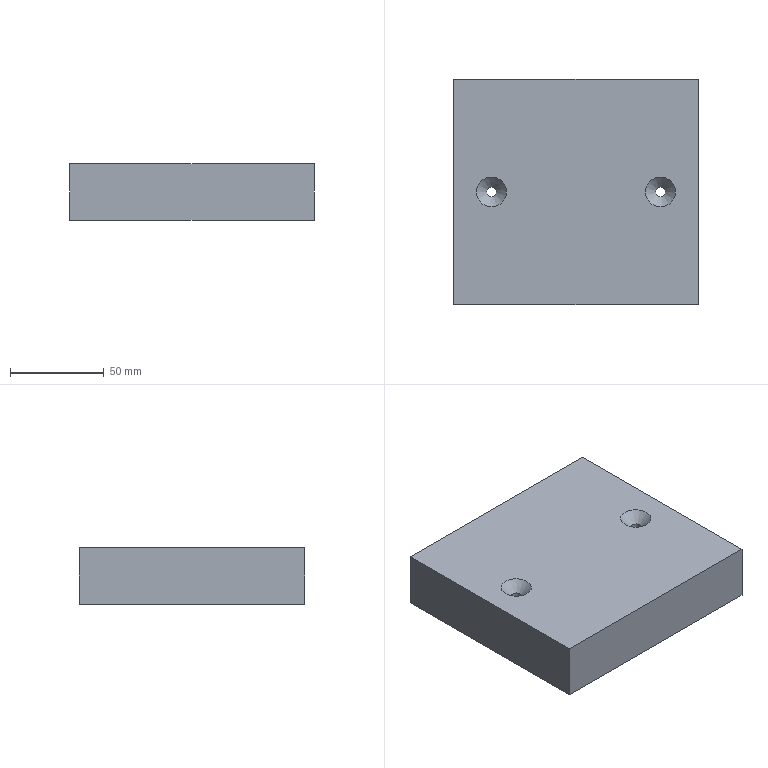Part | STEP file | YBQDJ-YY-5 | 1 solid | 10 faces | box 130 x 120 x 30 mm | volume 465920 mm3 | plane 6 | cylinder 2 | cone 2 | commonest cylinder face diameters 5.2 x2
STEP:
#1=CARTESIAN_POINT('',(0.,0.,0.));
#2=DIRECTION('',(0.,0.,1.));
#3=DIRECTION('',(1.,0.,0.));
#4=AXIS2_PLACEMENT_3D('',#1,#2,#3);
#5=CARTESIAN_POINT('',(168.9,305.,150.));
#6=VERTEX_POINT('',#5);
#7=CARTESIAN_POINT('',(171.5,305.,150.));
#8=DIRECTION('',(0.,0.,-1.));
#9=DIRECTION('',(-1.,0.,0.));
#10=AXIS2_PLACEMENT_3D('',#7,#8,#9);
#11=CIRCLE('',#10,2.6);
#12=CARTESIAN_POINT('',(171.5,305.,200.5));
#13=DIRECTION('',(0.,0.,-1.));
#14=DIRECTION('',(1.,0.,0.));
#15=AXIS2_PLACEMENT_3D('',#12,#13,#14);
#16=CYLINDRICAL_SURFACE('',#15,2.6);
#17=CARTESIAN_POINT('',(3.142,50.5));
#18=DIRECTION('',(1.,0.));
#19=VECTOR('',#18,1.);
#20=LINE('',#17,#19);
#21=(GEOMETRIC_REPRESENTATION_CONTEXT(2)PARAMETRIC_REPRESENTATION_CONTEXT()REPRESENTATION_CONTEXT('',''));
#22=DEFINITIONAL_REPRESENTATION('',(#20),#21);
#23=PCURVE('',#16,#22);
#24=CARTESIAN_POINT('',(251.5,412.,150.));
#25=DIRECTION('',(0.,0.,-1.));
#26=DIRECTION('',(-1.,0.,0.));
#27=AXIS2_PLACEMENT_3D('',#24,#25,#26);
#28=PLANE('',#27);
#29=CARTESIAN_POINT('',(80.,-107.));
#30=DIRECTION('',(1.,0.));
#31=AXIS2_PLACEMENT_2D('',#29,#30);
#32=CIRCLE('',#31,2.6);
#33=(GEOMETRIC_REPRESENTATION_CONTEXT(2)PARAMETRIC_REPRESENTATION_CONTEXT()REPRESENTATION_CONTEXT('',''));
#34=DEFINITIONAL_REPRESENTATION('',(#32),#33);
#35=PCURVE('',#28,#34);
#36=SURFACE_CURVE('',#11,(#23,#35),.PCURVE_S1.);
#37=EDGE_CURVE('',#6,#6,#36,.T.);
#38=ORIENTED_EDGE('',*,*,#37,.F.);
#39=CARTESIAN_POINT('',(168.9,305.,174.6));
#40=VERTEX_POINT('',#39);
#41=CARTESIAN_POINT('',(168.9,305.,174.6));
#42=CARTESIAN_POINT('',(168.9,305.,150.));
#43=B_SPLINE_CURVE_WITH_KNOTS('',1,(#41,#42),.UNSPECIFIED.,.F.,.F.,(2,2),(25.9,50.5),.PIECEWISE_BEZIER_KNOTS.);
#44=CARTESIAN_POINT('',(3.142,0.));
#45=DIRECTION('',(0.,1.));
#46=VECTOR('',#45,1.);
#47=LINE('',#44,#46);
#48=(GEOMETRIC_REPRESENTATION_CONTEXT(2)PARAMETRIC_REPRESENTATION_CONTEXT()REPRESENTATION_CONTEXT('',''));
#49=DEFINITIONAL_REPRESENTATION('',(#47),#48);
#50=PCURVE('',#16,#49);
#51=CARTESIAN_POINT('',(9.425,0.));
#52=DIRECTION('',(0.,1.));
#53=VECTOR('',#52,1.);
#54=LINE('',#51,#53);
#55=(GEOMETRIC_REPRESENTATION_CONTEXT(2)PARAMETRIC_REPRESENTATION_CONTEXT()REPRESENTATION_CONTEXT('',''));
#56=DEFINITIONAL_REPRESENTATION('',(#54),#55);
#57=PCURVE('',#16,#56);
#58=SEAM_CURVE('',#43,(#50,#57),.PCURVE_S1.);
#59=EDGE_CURVE('',#40,#6,#58,.T.);
#60=ORIENTED_EDGE('',*,*,#59,.F.);
#61=CARTESIAN_POINT('',(171.5,305.,174.6));
#62=DIRECTION('',(0.,0.,1.));
#63=DIRECTION('',(-1.,0.,0.));
#64=AXIS2_PLACEMENT_3D('',#61,#62,#63);
#65=CIRCLE('',#64,2.6);
#66=CARTESIAN_POINT('',(9.425,25.9));
#67=DIRECTION('',(-1.,0.));
#68=VECTOR('',#67,1.);
#69=LINE('',#66,#68);
#70=(GEOMETRIC_REPRESENTATION_CONTEXT(2)PARAMETRIC_REPRESENTATION_CONTEXT()REPRESENTATION_CONTEXT('',''));
#71=DEFINITIONAL_REPRESENTATION('',(#69),#70);
#72=PCURVE('',#16,#71);
#73=CARTESIAN_POINT('',(171.5,305.,175.));
#74=DIRECTION('',(0.,0.,1.));
#75=DIRECTION('',(-1.,0.,0.));
#76=AXIS2_PLACEMENT_3D('',#73,#74,#75);
#77=CONICAL_SURFACE('',#76,3.,0.7854);
#78=CARTESIAN_POINT('',(0.,-0.4));
#79=DIRECTION('',(1.,0.));
#80=VECTOR('',#79,1.);
#81=LINE('',#78,#80);
#82=(GEOMETRIC_REPRESENTATION_CONTEXT(2)PARAMETRIC_REPRESENTATION_CONTEXT()REPRESENTATION_CONTEXT('',''));
#83=DEFINITIONAL_REPRESENTATION('',(#81),#82);
#84=PCURVE('',#77,#83);
#85=SURFACE_CURVE('',#65,(#72,#84),.PCURVE_S1.);
#86=EDGE_CURVE('',#40,#40,#85,.T.);
#87=ORIENTED_EDGE('',*,*,#86,.F.);
#88=ORIENTED_EDGE('',*,*,#59,.T.);
#89=EDGE_LOOP('',(#38,#60,#87,#88));
#90=FACE_BOUND('',#89,.F.);
#91=ADVANCED_FACE('',(#90),#16,.F.);
#92=ORIENTED_EDGE('',*,*,#86,.T.);
#93=CARTESIAN_POINT('',(163.5,305.,180.));
#94=VERTEX_POINT('',#93);
#95=CARTESIAN_POINT('',(168.9,305.,174.6));
#96=CARTESIAN_POINT('',(163.5,305.,180.));
#97=B_SPLINE_CURVE_WITH_KNOTS('',1,(#95,#96),.UNSPECIFIED.,.F.,.F.,(2,2),(-0.5657,7.071),.PIECEWISE_BEZIER_KNOTS.);
#98=CARTESIAN_POINT('',(6.283,0.));
#99=DIRECTION('',(0.,1.));
#100=VECTOR('',#99,1.);
#101=LINE('',#98,#100);
#102=(GEOMETRIC_REPRESENTATION_CONTEXT(2)PARAMETRIC_REPRESENTATION_CONTEXT()REPRESENTATION_CONTEXT('',''));
#103=DEFINITIONAL_REPRESENTATION('',(#101),#102);
#104=PCURVE('',#77,#103);
#105=CARTESIAN_POINT('',(0.,0.));
#106=DIRECTION('',(0.,1.));
#107=VECTOR('',#106,1.);
#108=LINE('',#105,#107);
#109=(GEOMETRIC_REPRESENTATION_CONTEXT(2)PARAMETRIC_REPRESENTATION_CONTEXT()REPRESENTATION_CONTEXT('',''));
#110=DEFINITIONAL_REPRESENTATION('',(#108),#109);
#111=PCURVE('',#77,#110);
#112=SEAM_CURVE('',#97,(#104,#111),.PCURVE_S1.);
#113=EDGE_CURVE('',#40,#94,#112,.T.);
#114=ORIENTED_EDGE('',*,*,#113,.T.);
#115=CARTESIAN_POINT('',(179.5,305.,180.));
#116=VERTEX_POINT('',#115);
#117=CARTESIAN_POINT('',(171.5,305.,180.));
#118=DIRECTION('',(0.,0.,-1.));
#119=DIRECTION('',(1.,0.,0.));
#120=AXIS2_PLACEMENT_3D('',#117,#118,#119);
#121=CIRCLE('',#120,8.);
#122=CARTESIAN_POINT('',(9.425,5.));
#123=DIRECTION('',(-1.,0.));
#124=VECTOR('',#123,1.);
#125=LINE('',#122,#124);
#126=(GEOMETRIC_REPRESENTATION_CONTEXT(2)PARAMETRIC_REPRESENTATION_CONTEXT()REPRESENTATION_CONTEXT('',''));
#127=DEFINITIONAL_REPRESENTATION('',(#125),#126);
#128=PCURVE('',#77,#127);
#129=CARTESIAN_POINT('',(-49.497,0.,180.));
#130=DIRECTION('',(0.,0.,1.));
#131=DIRECTION('',(1.,0.,0.));
#132=AXIS2_PLACEMENT_3D('',#129,#130,#131);
#133=PLANE('',#132);
#134=CARTESIAN_POINT('',(228.997,305.));
#135=CARTESIAN_POINT('',(228.997,291.144));
#136=CARTESIAN_POINT('',(216.997,298.072));
#137=CARTESIAN_POINT('',(204.997,305.));
#138=CARTESIAN_POINT('',(216.997,311.928));
#139=CARTESIAN_POINT('',(228.997,318.856));
#140=CARTESIAN_POINT('',(228.997,305.));
#141=(BOUNDED_CURVE()B_SPLINE_CURVE(2,(#134,#135,#136,#137,#138,#139,#140),.UNSPECIFIED.,.T.,.F.)B_SPLINE_CURVE_WITH_KNOTS((1,2,2,2,2,1),(-2.094,0.,2.094,4.189,6.283,8.378),.UNSPECIFIED.)CURVE()GEOMETRIC_REPRESENTATION_ITEM()RATIONAL_B_SPLINE_CURVE((1.,0.5,1.,0.5,1.,0.5,1.))REPRESENTATION_ITEM(''));
#142=(GEOMETRIC_REPRESENTATION_CONTEXT(2)PARAMETRIC_REPRESENTATION_CONTEXT()REPRESENTATION_CONTEXT('',''));
#143=DEFINITIONAL_REPRESENTATION('',(#141),#142);
#144=PCURVE('',#133,#143);
#145=SURFACE_CURVE('',#121,(#128,#144),.PCURVE_S1.);
#146=EDGE_CURVE('',#94,#116,#145,.T.);
#147=ORIENTED_EDGE('',*,*,#146,.T.);
#148=CARTESIAN_POINT('',(171.5,305.,180.));
#149=DIRECTION('',(0.,0.,-1.));
#150=DIRECTION('',(1.,0.,0.));
#151=AXIS2_PLACEMENT_3D('',#148,#149,#150);
#152=CIRCLE('',#151,8.);
#153=CARTESIAN_POINT('',(3.142,5.));
#154=DIRECTION('',(-1.,0.));
#155=VECTOR('',#154,1.);
#156=LINE('',#153,#155);
#157=(GEOMETRIC_REPRESENTATION_CONTEXT(2)PARAMETRIC_REPRESENTATION_CONTEXT()REPRESENTATION_CONTEXT('',''));
#158=DEFINITIONAL_REPRESENTATION('',(#156),#157);
#159=PCURVE('',#77,#158);
#160=CARTESIAN_POINT('',(228.997,305.));
#161=CARTESIAN_POINT('',(228.997,291.144));
#162=CARTESIAN_POINT('',(216.997,298.072));
#163=CARTESIAN_POINT('',(204.997,305.));
#164=CARTESIAN_POINT('',(216.997,311.928));
#165=CARTESIAN_POINT('',(228.997,318.856));
#166=CARTESIAN_POINT('',(228.997,305.));
#167=(BOUNDED_CURVE()B_SPLINE_CURVE(2,(#160,#161,#162,#163,#164,#165,#166),.UNSPECIFIED.,.T.,.F.)B_SPLINE_CURVE_WITH_KNOTS((1,2,2,2,2,1),(-2.094,0.,2.094,4.189,6.283,8.378),.UNSPECIFIED.)CURVE()GEOMETRIC_REPRESENTATION_ITEM()RATIONAL_B_SPLINE_CURVE((1.,0.5,1.,0.5,1.,0.5,1.))REPRESENTATION_ITEM(''));
#168=(GEOMETRIC_REPRESENTATION_CONTEXT(2)PARAMETRIC_REPRESENTATION_CONTEXT()REPRESENTATION_CONTEXT('',''));
#169=DEFINITIONAL_REPRESENTATION('',(#167),#168);
#170=PCURVE('',#133,#169);
#171=SURFACE_CURVE('',#152,(#159,#170),.PCURVE_S1.);
#172=EDGE_CURVE('',#116,#94,#171,.T.);
#173=ORIENTED_EDGE('',*,*,#172,.T.);
#174=ORIENTED_EDGE('',*,*,#113,.F.);
#175=EDGE_LOOP('',(#92,#114,#147,#173,#174));
#176=FACE_BOUND('',#175,.F.);
#177=ADVANCED_FACE('',(#176),#77,.F.);
#178=CARTESIAN_POINT('',(258.9,305.,150.));
#179=VERTEX_POINT('',#178);
#180=CARTESIAN_POINT('',(261.5,305.,150.));
#181=DIRECTION('',(0.,0.,-1.));
#182=DIRECTION('',(-1.,0.,0.));
#183=AXIS2_PLACEMENT_3D('',#180,#181,#182);
#184=CIRCLE('',#183,2.6);
#185=CARTESIAN_POINT('',(261.5,305.,200.5));
#186=DIRECTION('',(0.,0.,-1.));
#187=DIRECTION('',(-1.,0.,0.));
#188=AXIS2_PLACEMENT_3D('',#185,#186,#187);
#189=CYLINDRICAL_SURFACE('',#188,2.6);
#190=CARTESIAN_POINT('',(0.,50.5));
#191=DIRECTION('',(1.,0.));
#192=VECTOR('',#191,1.);
#193=LINE('',#190,#192);
#194=(GEOMETRIC_REPRESENTATION_CONTEXT(2)PARAMETRIC_REPRESENTATION_CONTEXT()REPRESENTATION_CONTEXT('',''));
#195=DEFINITIONAL_REPRESENTATION('',(#193),#194);
#196=PCURVE('',#189,#195);
#197=CARTESIAN_POINT('',(-10.,-107.));
#198=DIRECTION('',(1.,0.));
#199=AXIS2_PLACEMENT_2D('',#197,#198);
#200=CIRCLE('',#199,2.6);
#201=(GEOMETRIC_REPRESENTATION_CONTEXT(2)PARAMETRIC_REPRESENTATION_CONTEXT()REPRESENTATION_CONTEXT('',''));
#202=DEFINITIONAL_REPRESENTATION('',(#200),#201);
#203=PCURVE('',#28,#202);
#204=SURFACE_CURVE('',#184,(#196,#203),.PCURVE_S1.);
#205=EDGE_CURVE('',#179,#179,#204,.T.);
#206=ORIENTED_EDGE('',*,*,#205,.F.);
#207=CARTESIAN_POINT('',(258.9,305.,174.6));
#208=VERTEX_POINT('',#207);
#209=CARTESIAN_POINT('',(258.9,305.,174.6));
#210=CARTESIAN_POINT('',(258.9,305.,150.));
#211=B_SPLINE_CURVE_WITH_KNOTS('',1,(#209,#210),.UNSPECIFIED.,.F.,.F.,(2,2),(25.9,50.5),.PIECEWISE_BEZIER_KNOTS.);
#212=CARTESIAN_POINT('',(0.,0.));
#213=DIRECTION('',(0.,1.));
#214=VECTOR('',#213,1.);
#215=LINE('',#212,#214);
#216=(GEOMETRIC_REPRESENTATION_CONTEXT(2)PARAMETRIC_REPRESENTATION_CONTEXT()REPRESENTATION_CONTEXT('',''));
#217=DEFINITIONAL_REPRESENTATION('',(#215),#216);
#218=PCURVE('',#189,#217);
#219=CARTESIAN_POINT('',(6.283,0.));
#220=DIRECTION('',(0.,1.));
#221=VECTOR('',#220,1.);
#222=LINE('',#219,#221);
#223=(GEOMETRIC_REPRESENTATION_CONTEXT(2)PARAMETRIC_REPRESENTATION_CONTEXT()REPRESENTATION_CONTEXT('',''));
#224=DEFINITIONAL_REPRESENTATION('',(#222),#223);
#225=PCURVE('',#189,#224);
#226=SEAM_CURVE('',#211,(#218,#225),.PCURVE_S1.);
#227=EDGE_CURVE('',#208,#179,#226,.T.);
#228=ORIENTED_EDGE('',*,*,#227,.F.);
#229=CARTESIAN_POINT('',(264.1,305.,174.6));
#230=VERTEX_POINT('',#229);
#231=CARTESIAN_POINT('',(261.5,305.,174.6));
#232=DIRECTION('',(0.,0.,1.));
#233=DIRECTION('',(1.,0.,0.));
#234=AXIS2_PLACEMENT_3D('',#231,#232,#233);
#235=CIRCLE('',#234,2.6);
#236=CARTESIAN_POINT('',(3.142,25.9));
#237=DIRECTION('',(-1.,0.));
#238=VECTOR('',#237,1.);
#239=LINE('',#236,#238);
#240=(GEOMETRIC_REPRESENTATION_CONTEXT(2)PARAMETRIC_REPRESENTATION_CONTEXT()REPRESENTATION_CONTEXT('',''));
#241=DEFINITIONAL_REPRESENTATION('',(#239),#240);
#242=PCURVE('',#189,#241);
#243=CARTESIAN_POINT('',(261.5,305.,175.));
#244=DIRECTION('',(0.,0.,1.));
#245=DIRECTION('',(1.,0.,0.));
#246=AXIS2_PLACEMENT_3D('',#243,#244,#245);
#247=CONICAL_SURFACE('',#246,3.,0.7854);
#248=CARTESIAN_POINT('',(0.,-0.4));
#249=DIRECTION('',(1.,0.));
#250=VECTOR('',#249,1.);
#251=LINE('',#248,#250);
#252=(GEOMETRIC_REPRESENTATION_CONTEXT(2)PARAMETRIC_REPRESENTATION_CONTEXT()REPRESENTATION_CONTEXT('',''));
#253=DEFINITIONAL_REPRESENTATION('',(#251),#252);
#254=PCURVE('',#247,#253);
#255=SURFACE_CURVE('',#235,(#242,#254),.PCURVE_S1.);
#256=EDGE_CURVE('',#230,#208,#255,.T.);
#257=ORIENTED_EDGE('',*,*,#256,.F.);
#258=CARTESIAN_POINT('',(261.5,305.,174.6));
#259=DIRECTION('',(0.,0.,1.));
#260=DIRECTION('',(1.,0.,0.));
#261=AXIS2_PLACEMENT_3D('',#258,#259,#260);
#262=CIRCLE('',#261,2.6);
#263=CARTESIAN_POINT('',(9.425,25.9));
#264=DIRECTION('',(-1.,0.));
#265=VECTOR('',#264,1.);
#266=LINE('',#263,#265);
#267=(GEOMETRIC_REPRESENTATION_CONTEXT(2)PARAMETRIC_REPRESENTATION_CONTEXT()REPRESENTATION_CONTEXT('',''));
#268=DEFINITIONAL_REPRESENTATION('',(#266),#267);
#269=PCURVE('',#189,#268);
#270=CARTESIAN_POINT('',(0.,-0.4));
#271=DIRECTION('',(1.,0.));
#272=VECTOR('',#271,1.);
#273=LINE('',#270,#272);
#274=(GEOMETRIC_REPRESENTATION_CONTEXT(2)PARAMETRIC_REPRESENTATION_CONTEXT()REPRESENTATION_CONTEXT('',''));
#275=DEFINITIONAL_REPRESENTATION('',(#273),#274);
#276=PCURVE('',#247,#275);
#277=SURFACE_CURVE('',#262,(#269,#276),.PCURVE_S1.);
#278=EDGE_CURVE('',#208,#230,#277,.T.);
#279=ORIENTED_EDGE('',*,*,#278,.F.);
#280=ORIENTED_EDGE('',*,*,#227,.T.);
#281=EDGE_LOOP('',(#206,#228,#257,#279,#280));
#282=FACE_BOUND('',#281,.F.);
#283=ADVANCED_FACE('',(#282),#189,.F.);
#284=CARTESIAN_POINT('',(281.5,365.,180.));
#285=VERTEX_POINT('',#284);
#286=CARTESIAN_POINT('',(151.5,365.,180.));
#287=VERTEX_POINT('',#286);
#288=CARTESIAN_POINT('',(-49.497,365.,180.));
#289=DIRECTION('',(-1.,0.,0.));
#290=VECTOR('',#289,1.);
#291=LINE('',#288,#290);
#292=CARTESIAN_POINT('',(276.5,365.,157.5));
#293=DIRECTION('',(0.,1.,0.));
#294=DIRECTION('',(0.,0.,1.));
#295=AXIS2_PLACEMENT_3D('',#292,#293,#294);
#296=PLANE('',#295);
#297=CARTESIAN_POINT('',(22.5,-325.997));
#298=DIRECTION('',(0.,-1.));
#299=VECTOR('',#298,1.);
#300=LINE('',#297,#299);
#301=(GEOMETRIC_REPRESENTATION_CONTEXT(2)PARAMETRIC_REPRESENTATION_CONTEXT()REPRESENTATION_CONTEXT('',''));
#302=DEFINITIONAL_REPRESENTATION('',(#300),#301);
#303=PCURVE('',#296,#302);
#304=CARTESIAN_POINT('',(0.,365.));
#305=DIRECTION('',(-1.,0.));
#306=VECTOR('',#305,1.);
#307=LINE('',#304,#306);
#308=(GEOMETRIC_REPRESENTATION_CONTEXT(2)PARAMETRIC_REPRESENTATION_CONTEXT()REPRESENTATION_CONTEXT('',''));
#309=DEFINITIONAL_REPRESENTATION('',(#307),#308);
#310=PCURVE('',#133,#309);
#311=SURFACE_CURVE('',#291,(#303,#310),.PCURVE_S1.);
#312=EDGE_CURVE('',#285,#287,#311,.T.);
#313=ORIENTED_EDGE('',*,*,#312,.F.);
#314=CARTESIAN_POINT('',(281.5,365.,150.));
#315=VERTEX_POINT('',#314);
#316=CARTESIAN_POINT('',(281.5,365.,185.));
#317=DIRECTION('',(0.,0.,1.));
#318=VECTOR('',#317,1.);
#319=LINE('',#316,#318);
#320=CARTESIAN_POINT('',(27.5,5.));
#321=DIRECTION('',(1.,0.));
#322=VECTOR('',#321,1.);
#323=LINE('',#320,#322);
#324=(GEOMETRIC_REPRESENTATION_CONTEXT(2)PARAMETRIC_REPRESENTATION_CONTEXT()REPRESENTATION_CONTEXT('',''));
#325=DEFINITIONAL_REPRESENTATION('',(#323),#324);
#326=PCURVE('',#296,#325);
#327=CARTESIAN_POINT('',(281.5,210.,185.));
#328=DIRECTION('',(-1.,0.,0.));
#329=DIRECTION('',(0.,-1.,0.));
#330=AXIS2_PLACEMENT_3D('',#327,#328,#329);
#331=PLANE('',#330);
#332=CARTESIAN_POINT('',(-155.,0.));
#333=DIRECTION('',(0.,1.));
#334=VECTOR('',#333,1.);
#335=LINE('',#332,#334);
#336=(GEOMETRIC_REPRESENTATION_CONTEXT(2)PARAMETRIC_REPRESENTATION_CONTEXT()REPRESENTATION_CONTEXT('',''));
#337=DEFINITIONAL_REPRESENTATION('',(#335),#336);
#338=PCURVE('',#331,#337);
#339=SURFACE_CURVE('',#319,(#326,#338),.PCURVE_S1.);
#340=EDGE_CURVE('',#315,#285,#339,.T.);
#341=ORIENTED_EDGE('',*,*,#340,.F.);
#342=CARTESIAN_POINT('',(151.5,365.,150.));
#343=VERTEX_POINT('',#342);
#344=CARTESIAN_POINT('',(276.5,365.,150.));
#345=DIRECTION('',(-1.,0.,0.));
#346=VECTOR('',#345,1.);
#347=LINE('',#344,#346);
#348=CARTESIAN_POINT('',(-7.5,0.));
#349=DIRECTION('',(0.,-1.));
#350=VECTOR('',#349,1.);
#351=LINE('',#348,#350);
#352=(GEOMETRIC_REPRESENTATION_CONTEXT(2)PARAMETRIC_REPRESENTATION_CONTEXT()REPRESENTATION_CONTEXT('',''));
#353=DEFINITIONAL_REPRESENTATION('',(#351),#352);
#354=PCURVE('',#296,#353);
#355=CARTESIAN_POINT('',(-25.,-47.));
#356=DIRECTION('',(1.,0.));
#357=VECTOR('',#356,1.);
#358=LINE('',#355,#357);
#359=(GEOMETRIC_REPRESENTATION_CONTEXT(2)PARAMETRIC_REPRESENTATION_CONTEXT()REPRESENTATION_CONTEXT('',''));
#360=DEFINITIONAL_REPRESENTATION('',(#358),#359);
#361=PCURVE('',#28,#360);
#362=SURFACE_CURVE('',#347,(#354,#361),.PCURVE_S1.);
#363=EDGE_CURVE('',#315,#343,#362,.T.);
#364=ORIENTED_EDGE('',*,*,#363,.T.);
#365=CARTESIAN_POINT('',(151.5,365.,157.5));
#366=DIRECTION('',(0.,0.,1.));
#367=VECTOR('',#366,1.);
#368=LINE('',#365,#367);
#369=CARTESIAN_POINT('',(0.,-125.));
#370=DIRECTION('',(1.,0.));
#371=VECTOR('',#370,1.);
#372=LINE('',#369,#371);
#373=(GEOMETRIC_REPRESENTATION_CONTEXT(2)PARAMETRIC_REPRESENTATION_CONTEXT()REPRESENTATION_CONTEXT('',''));
#374=DEFINITIONAL_REPRESENTATION('',(#372),#373);
#375=PCURVE('',#296,#374);
#376=CARTESIAN_POINT('',(151.5,400.,185.));
#377=DIRECTION('',(1.,0.,0.));
#378=DIRECTION('',(0.,0.,-1.));
#379=AXIS2_PLACEMENT_3D('',#376,#377,#378);
#380=PLANE('',#379);
#381=CARTESIAN_POINT('',(27.5,-35.));
#382=DIRECTION('',(-1.,0.));
#383=VECTOR('',#382,1.);
#384=LINE('',#381,#383);
#385=(GEOMETRIC_REPRESENTATION_CONTEXT(2)PARAMETRIC_REPRESENTATION_CONTEXT()REPRESENTATION_CONTEXT('',''));
#386=DEFINITIONAL_REPRESENTATION('',(#384),#385);
#387=PCURVE('',#380,#386);
#388=SURFACE_CURVE('',#368,(#375,#387),.PCURVE_S1.);
#389=EDGE_CURVE('',#343,#287,#388,.T.);
#390=ORIENTED_EDGE('',*,*,#389,.T.);
#391=EDGE_LOOP('',(#313,#341,#364,#390));
#392=FACE_BOUND('',#391,.T.);
#393=ADVANCED_FACE('',(#392),#296,.T.);
#394=CARTESIAN_POINT('',(281.5,245.,180.));
#395=VERTEX_POINT('',#394);
#396=CARTESIAN_POINT('',(281.5,0.,180.));
#397=DIRECTION('',(0.,1.,0.));
#398=VECTOR('',#397,1.);
#399=LINE('',#396,#398);
#400=CARTESIAN_POINT('',(210.,-5.));
#401=DIRECTION('',(-1.,0.));
#402=VECTOR('',#401,1.);
#403=LINE('',#400,#402);
#404=(GEOMETRIC_REPRESENTATION_CONTEXT(2)PARAMETRIC_REPRESENTATION_CONTEXT()REPRESENTATION_CONTEXT('',''));
#405=DEFINITIONAL_REPRESENTATION('',(#403),#404);
#406=PCURVE('',#331,#405);
#407=CARTESIAN_POINT('',(330.997,0.));
#408=DIRECTION('',(0.,1.));
#409=VECTOR('',#408,1.);
#410=LINE('',#407,#409);
#411=(GEOMETRIC_REPRESENTATION_CONTEXT(2)PARAMETRIC_REPRESENTATION_CONTEXT()REPRESENTATION_CONTEXT('',''));
#412=DEFINITIONAL_REPRESENTATION('',(#410),#411);
#413=PCURVE('',#133,#412);
#414=SURFACE_CURVE('',#399,(#406,#413),.PCURVE_S1.);
#415=EDGE_CURVE('',#395,#285,#414,.T.);
#416=ORIENTED_EDGE('',*,*,#415,.F.);
#417=CARTESIAN_POINT('',(281.5,245.,150.));
#418=VERTEX_POINT('',#417);
#419=CARTESIAN_POINT('',(281.5,245.,157.5));
#420=DIRECTION('',(0.,0.,1.));
#421=VECTOR('',#420,1.);
#422=LINE('',#419,#421);
#423=CARTESIAN_POINT('',(-35.,-27.5));
#424=DIRECTION('',(0.,1.));
#425=VECTOR('',#424,1.);
#426=LINE('',#423,#425);
#427=(GEOMETRIC_REPRESENTATION_CONTEXT(2)PARAMETRIC_REPRESENTATION_CONTEXT()REPRESENTATION_CONTEXT('',''));
#428=DEFINITIONAL_REPRESENTATION('',(#426),#427);
#429=PCURVE('',#331,#428);
#430=CARTESIAN_POINT('',(156.5,245.,157.5));
#431=DIRECTION('',(0.,-1.,0.));
#432=DIRECTION('',(0.,0.,-1.));
#433=AXIS2_PLACEMENT_3D('',#430,#431,#432);
#434=PLANE('',#433);
#435=CARTESIAN_POINT('',(0.,125.));
#436=DIRECTION('',(-1.,0.));
#437=VECTOR('',#436,1.);
#438=LINE('',#435,#437);
#439=(GEOMETRIC_REPRESENTATION_CONTEXT(2)PARAMETRIC_REPRESENTATION_CONTEXT()REPRESENTATION_CONTEXT('',''));
#440=DEFINITIONAL_REPRESENTATION('',(#438),#439);
#441=PCURVE('',#434,#440);
#442=SURFACE_CURVE('',#422,(#429,#441),.PCURVE_S1.);
#443=EDGE_CURVE('',#418,#395,#442,.T.);
#444=ORIENTED_EDGE('',*,*,#443,.F.);
#445=CARTESIAN_POINT('',(281.5,210.,150.));
#446=DIRECTION('',(0.,1.,0.));
#447=VECTOR('',#446,1.);
#448=LINE('',#445,#447);
#449=CARTESIAN_POINT('',(0.,-35.));
#450=DIRECTION('',(-1.,0.));
#451=VECTOR('',#450,1.);
#452=LINE('',#449,#451);
#453=(GEOMETRIC_REPRESENTATION_CONTEXT(2)PARAMETRIC_REPRESENTATION_CONTEXT()REPRESENTATION_CONTEXT('',''));
#454=DEFINITIONAL_REPRESENTATION('',(#452),#453);
#455=PCURVE('',#331,#454);
#456=CARTESIAN_POINT('',(-30.,-202.));
#457=DIRECTION('',(0.,1.));
#458=VECTOR('',#457,1.);
#459=LINE('',#456,#458);
#460=(GEOMETRIC_REPRESENTATION_CONTEXT(2)PARAMETRIC_REPRESENTATION_CONTEXT()REPRESENTATION_CONTEXT('',''));
#461=DEFINITIONAL_REPRESENTATION('',(#459),#460);
#462=PCURVE('',#28,#461);
#463=SURFACE_CURVE('',#448,(#455,#462),.PCURVE_S1.);
#464=EDGE_CURVE('',#418,#315,#463,.T.);
#465=ORIENTED_EDGE('',*,*,#464,.T.);
#466=ORIENTED_EDGE('',*,*,#340,.T.);
#467=EDGE_LOOP('',(#416,#444,#465,#466));
#468=FACE_BOUND('',#467,.T.);
#469=ADVANCED_FACE('',(#468),#331,.F.);
#470=CARTESIAN_POINT('',(151.5,245.,180.));
#471=VERTEX_POINT('',#470);
#472=CARTESIAN_POINT('',(-49.497,245.,180.));
#473=DIRECTION('',(1.,0.,0.));
#474=VECTOR('',#473,1.);
#475=LINE('',#472,#474);
#476=CARTESIAN_POINT('',(-22.5,-205.997));
#477=DIRECTION('',(0.,1.));
#478=VECTOR('',#477,1.);
#479=LINE('',#476,#478);
#480=(GEOMETRIC_REPRESENTATION_CONTEXT(2)PARAMETRIC_REPRESENTATION_CONTEXT()REPRESENTATION_CONTEXT('',''));
#481=DEFINITIONAL_REPRESENTATION('',(#479),#480);
#482=PCURVE('',#434,#481);
#483=CARTESIAN_POINT('',(0.,245.));
#484=DIRECTION('',(1.,0.));
#485=VECTOR('',#484,1.);
#486=LINE('',#483,#485);
#487=(GEOMETRIC_REPRESENTATION_CONTEXT(2)PARAMETRIC_REPRESENTATION_CONTEXT()REPRESENTATION_CONTEXT('',''));
#488=DEFINITIONAL_REPRESENTATION('',(#486),#487);
#489=PCURVE('',#133,#488);
#490=SURFACE_CURVE('',#475,(#482,#489),.PCURVE_S1.);
#491=EDGE_CURVE('',#471,#395,#490,.T.);
#492=ORIENTED_EDGE('',*,*,#491,.F.);
#493=CARTESIAN_POINT('',(151.5,245.,150.));
#494=VERTEX_POINT('',#493);
#495=CARTESIAN_POINT('',(151.5,245.,185.));
#496=DIRECTION('',(0.,0.,1.));
#497=VECTOR('',#496,1.);
#498=LINE('',#495,#497);
#499=CARTESIAN_POINT('',(-27.5,-5.));
#500=DIRECTION('',(-1.,0.));
#501=VECTOR('',#500,1.);
#502=LINE('',#499,#501);
#503=(GEOMETRIC_REPRESENTATION_CONTEXT(2)PARAMETRIC_REPRESENTATION_CONTEXT()REPRESENTATION_CONTEXT('',''));
#504=DEFINITIONAL_REPRESENTATION('',(#502),#503);
#505=PCURVE('',#434,#504);
#506=CARTESIAN_POINT('',(0.,-155.));
#507=DIRECTION('',(-1.,0.));
#508=VECTOR('',#507,1.);
#509=LINE('',#506,#508);
#510=(GEOMETRIC_REPRESENTATION_CONTEXT(2)PARAMETRIC_REPRESENTATION_CONTEXT()REPRESENTATION_CONTEXT('',''));
#511=DEFINITIONAL_REPRESENTATION('',(#509),#510);
#512=PCURVE('',#380,#511);
#513=SURFACE_CURVE('',#498,(#505,#512),.PCURVE_S1.);
#514=EDGE_CURVE('',#494,#471,#513,.T.);
#515=ORIENTED_EDGE('',*,*,#514,.F.);
#516=CARTESIAN_POINT('',(156.5,245.,150.));
#517=DIRECTION('',(1.,0.,0.));
#518=VECTOR('',#517,1.);
#519=LINE('',#516,#518);
#520=CARTESIAN_POINT('',(7.5,0.));
#521=DIRECTION('',(0.,1.));
#522=VECTOR('',#521,1.);
#523=LINE('',#520,#522);
#524=(GEOMETRIC_REPRESENTATION_CONTEXT(2)PARAMETRIC_REPRESENTATION_CONTEXT()REPRESENTATION_CONTEXT('',''));
#525=DEFINITIONAL_REPRESENTATION('',(#523),#524);
#526=PCURVE('',#434,#525);
#527=CARTESIAN_POINT('',(95.,-167.));
#528=DIRECTION('',(-1.,0.));
#529=VECTOR('',#528,1.);
#530=LINE('',#527,#529);
#531=(GEOMETRIC_REPRESENTATION_CONTEXT(2)PARAMETRIC_REPRESENTATION_CONTEXT()REPRESENTATION_CONTEXT('',''));
#532=DEFINITIONAL_REPRESENTATION('',(#530),#531);
#533=PCURVE('',#28,#532);
#534=SURFACE_CURVE('',#519,(#526,#533),.PCURVE_S1.);
#535=EDGE_CURVE('',#494,#418,#534,.T.);
#536=ORIENTED_EDGE('',*,*,#535,.T.);
#537=ORIENTED_EDGE('',*,*,#443,.T.);
#538=EDGE_LOOP('',(#492,#515,#536,#537));
#539=FACE_BOUND('',#538,.T.);
#540=ADVANCED_FACE('',(#539),#434,.T.);
#541=CARTESIAN_POINT('',(151.5,0.,180.));
#542=DIRECTION('',(0.,-1.,0.));
#543=VECTOR('',#542,1.);
#544=LINE('',#541,#543);
#545=CARTESIAN_POINT('',(5.,-400.));
#546=DIRECTION('',(0.,-1.));
#547=VECTOR('',#546,1.);
#548=LINE('',#545,#547);
#549=(GEOMETRIC_REPRESENTATION_CONTEXT(2)PARAMETRIC_REPRESENTATION_CONTEXT()REPRESENTATION_CONTEXT('',''));
#550=DEFINITIONAL_REPRESENTATION('',(#548),#549);
#551=PCURVE('',#380,#550);
#552=CARTESIAN_POINT('',(200.997,0.));
#553=DIRECTION('',(0.,-1.));
#554=VECTOR('',#553,1.);
#555=LINE('',#552,#554);
#556=(GEOMETRIC_REPRESENTATION_CONTEXT(2)PARAMETRIC_REPRESENTATION_CONTEXT()REPRESENTATION_CONTEXT('',''));
#557=DEFINITIONAL_REPRESENTATION('',(#555),#556);
#558=PCURVE('',#133,#557);
#559=SURFACE_CURVE('',#544,(#551,#558),.PCURVE_S1.);
#560=EDGE_CURVE('',#287,#471,#559,.T.);
#561=ORIENTED_EDGE('',*,*,#560,.F.);
#562=ORIENTED_EDGE('',*,*,#389,.F.);
#563=CARTESIAN_POINT('',(151.5,400.,150.));
#564=DIRECTION('',(0.,-1.,0.));
#565=VECTOR('',#564,1.);
#566=LINE('',#563,#565);
#567=CARTESIAN_POINT('',(35.,0.));
#568=DIRECTION('',(0.,-1.));
#569=VECTOR('',#568,1.);
#570=LINE('',#567,#569);
#571=(GEOMETRIC_REPRESENTATION_CONTEXT(2)PARAMETRIC_REPRESENTATION_CONTEXT()REPRESENTATION_CONTEXT('',''));
#572=DEFINITIONAL_REPRESENTATION('',(#570),#571);
#573=PCURVE('',#380,#572);
#574=CARTESIAN_POINT('',(100.,-12.));
#575=DIRECTION('',(0.,-1.));
#576=VECTOR('',#575,1.);
#577=LINE('',#574,#576);
#578=(GEOMETRIC_REPRESENTATION_CONTEXT(2)PARAMETRIC_REPRESENTATION_CONTEXT()REPRESENTATION_CONTEXT('',''));
#579=DEFINITIONAL_REPRESENTATION('',(#577),#578);
#580=PCURVE('',#28,#579);
#581=SURFACE_CURVE('',#566,(#573,#580),.PCURVE_S1.);
#582=EDGE_CURVE('',#343,#494,#581,.T.);
#583=ORIENTED_EDGE('',*,*,#582,.T.);
#584=ORIENTED_EDGE('',*,*,#514,.T.);
#585=EDGE_LOOP('',(#561,#562,#583,#584));
#586=FACE_BOUND('',#585,.T.);
#587=ADVANCED_FACE('',(#586),#380,.F.);
#588=ORIENTED_EDGE('',*,*,#278,.T.);
#589=CARTESIAN_POINT('',(269.5,305.,180.));
#590=VERTEX_POINT('',#589);
#591=CARTESIAN_POINT('',(264.1,305.,174.6));
#592=CARTESIAN_POINT('',(269.5,305.,180.));
#593=B_SPLINE_CURVE_WITH_KNOTS('',1,(#591,#592),.UNSPECIFIED.,.F.,.F.,(2,2),(-0.5657,7.071),.PIECEWISE_BEZIER_KNOTS.);
#594=CARTESIAN_POINT('',(6.283,0.));
#595=DIRECTION('',(0.,1.));
#596=VECTOR('',#595,1.);
#597=LINE('',#594,#596);
#598=(GEOMETRIC_REPRESENTATION_CONTEXT(2)PARAMETRIC_REPRESENTATION_CONTEXT()REPRESENTATION_CONTEXT('',''));
#599=DEFINITIONAL_REPRESENTATION('',(#597),#598);
#600=PCURVE('',#247,#599);
#601=CARTESIAN_POINT('',(0.,0.));
#602=DIRECTION('',(0.,1.));
#603=VECTOR('',#602,1.);
#604=LINE('',#601,#603);
#605=(GEOMETRIC_REPRESENTATION_CONTEXT(2)PARAMETRIC_REPRESENTATION_CONTEXT()REPRESENTATION_CONTEXT('',''));
#606=DEFINITIONAL_REPRESENTATION('',(#604),#605);
#607=PCURVE('',#247,#606);
#608=SEAM_CURVE('',#593,(#600,#607),.PCURVE_S1.);
#609=EDGE_CURVE('',#230,#590,#608,.T.);
#610=ORIENTED_EDGE('',*,*,#609,.T.);
#611=CARTESIAN_POINT('',(261.5,305.,180.));
#612=DIRECTION('',(0.,0.,-1.));
#613=DIRECTION('',(1.,0.,0.));
#614=AXIS2_PLACEMENT_3D('',#611,#612,#613);
#615=CIRCLE('',#614,8.);
#616=CARTESIAN_POINT('',(6.283,5.));
#617=DIRECTION('',(-1.,0.));
#618=VECTOR('',#617,1.);
#619=LINE('',#616,#618);
#620=(GEOMETRIC_REPRESENTATION_CONTEXT(2)PARAMETRIC_REPRESENTATION_CONTEXT()REPRESENTATION_CONTEXT('',''));
#621=DEFINITIONAL_REPRESENTATION('',(#619),#620);
#622=PCURVE('',#247,#621);
#623=CARTESIAN_POINT('',(318.997,305.));
#624=CARTESIAN_POINT('',(318.997,291.144));
#625=CARTESIAN_POINT('',(306.997,298.072));
#626=CARTESIAN_POINT('',(294.997,305.));
#627=CARTESIAN_POINT('',(306.997,311.928));
#628=CARTESIAN_POINT('',(318.997,318.856));
#629=CARTESIAN_POINT('',(318.997,305.));
#630=(BOUNDED_CURVE()B_SPLINE_CURVE(2,(#623,#624,#625,#626,#627,#628,#629),.UNSPECIFIED.,.T.,.F.)B_SPLINE_CURVE_WITH_KNOTS((1,2,2,2,2,1),(-2.094,0.,2.094,4.189,6.283,8.378),.UNSPECIFIED.)CURVE()GEOMETRIC_REPRESENTATION_ITEM()RATIONAL_B_SPLINE_CURVE((1.,0.5,1.,0.5,1.,0.5,1.))REPRESENTATION_ITEM(''));
#631=(GEOMETRIC_REPRESENTATION_CONTEXT(2)PARAMETRIC_REPRESENTATION_CONTEXT()REPRESENTATION_CONTEXT('',''));
#632=DEFINITIONAL_REPRESENTATION('',(#630),#631);
#633=PCURVE('',#133,#632);
#634=SURFACE_CURVE('',#615,(#622,#633),.PCURVE_S1.);
#635=EDGE_CURVE('',#590,#590,#634,.T.);
#636=ORIENTED_EDGE('',*,*,#635,.T.);
#637=ORIENTED_EDGE('',*,*,#609,.F.);
#638=ORIENTED_EDGE('',*,*,#256,.T.);
#639=EDGE_LOOP('',(#588,#610,#636,#637,#638));
#640=FACE_BOUND('',#639,.F.);
#641=ADVANCED_FACE('',(#640),#247,.F.);
#642=ORIENTED_EDGE('',*,*,#172,.T.);
#643=ORIENTED_EDGE('',*,*,#146,.T.);
#644=EDGE_LOOP('',(#642,#643));
#645=FACE_BOUND('',#644,.T.);
#646=ORIENTED_EDGE('',*,*,#635,.T.);
#647=EDGE_LOOP('',(#646));
#648=FACE_BOUND('',#647,.T.);
#649=ORIENTED_EDGE('',*,*,#560,.T.);
#650=ORIENTED_EDGE('',*,*,#491,.T.);
#651=ORIENTED_EDGE('',*,*,#415,.T.);
#652=ORIENTED_EDGE('',*,*,#312,.T.);
#653=EDGE_LOOP('',(#649,#650,#651,#652));
#654=FACE_BOUND('',#653,.T.);
#655=ADVANCED_FACE('',(#645,#648,#654),#133,.T.);
#656=ORIENTED_EDGE('',*,*,#582,.F.);
#657=ORIENTED_EDGE('',*,*,#363,.F.);
#658=ORIENTED_EDGE('',*,*,#464,.F.);
#659=ORIENTED_EDGE('',*,*,#535,.F.);
#660=EDGE_LOOP('',(#656,#657,#658,#659));
#661=FACE_BOUND('',#660,.T.);
#662=ORIENTED_EDGE('',*,*,#37,.F.);
#663=EDGE_LOOP('',(#662));
#664=FACE_BOUND('',#663,.T.);
#665=ORIENTED_EDGE('',*,*,#205,.F.);
#666=EDGE_LOOP('',(#665));
#667=FACE_BOUND('',#666,.T.);
#668=ADVANCED_FACE('',(#661,#664,#667),#28,.T.);
#669=CLOSED_SHELL('',(#91,#177,#283,#393,#469,#540,#587,#641,#655,#668));
#670=MANIFOLD_SOLID_BREP('',#669);
#671=(LENGTH_UNIT()NAMED_UNIT(*)SI_UNIT(.MILLI.,.METRE.));
#672=UNCERTAINTY_MEASURE_WITH_UNIT(LENGTH_MEASURE(0.000005),#671,'','');
#673=(NAMED_UNIT(*)PLANE_ANGLE_UNIT()SI_UNIT($,.RADIAN.));
#674=(NAMED_UNIT(*)SI_UNIT($,.STERADIAN.)SOLID_ANGLE_UNIT());
#675=(GEOMETRIC_REPRESENTATION_CONTEXT(3)GLOBAL_UNCERTAINTY_ASSIGNED_CONTEXT((#672))GLOBAL_UNIT_ASSIGNED_CONTEXT((#671,#673,#674))REPRESENTATION_CONTEXT('',''));
#676=ADVANCED_BREP_SHAPE_REPRESENTATION('',(#4,#670),#675);